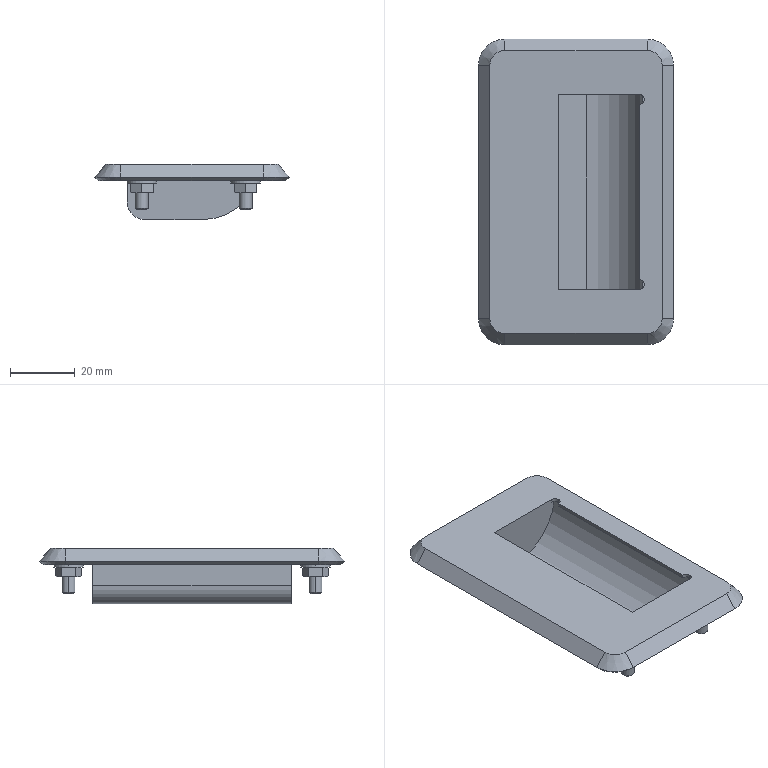Part | SolidWorks | features BaseBody 9 | 9 solids | 190 faces | box 60 x 94 x 17 mm | volume 17797 mm3 | cone 80 | plane 70 | cylinder 40 | commonest cylinder face diameters 3.242 x8 4 x8 4.2 x8 9 x8 3 x4 10 x1